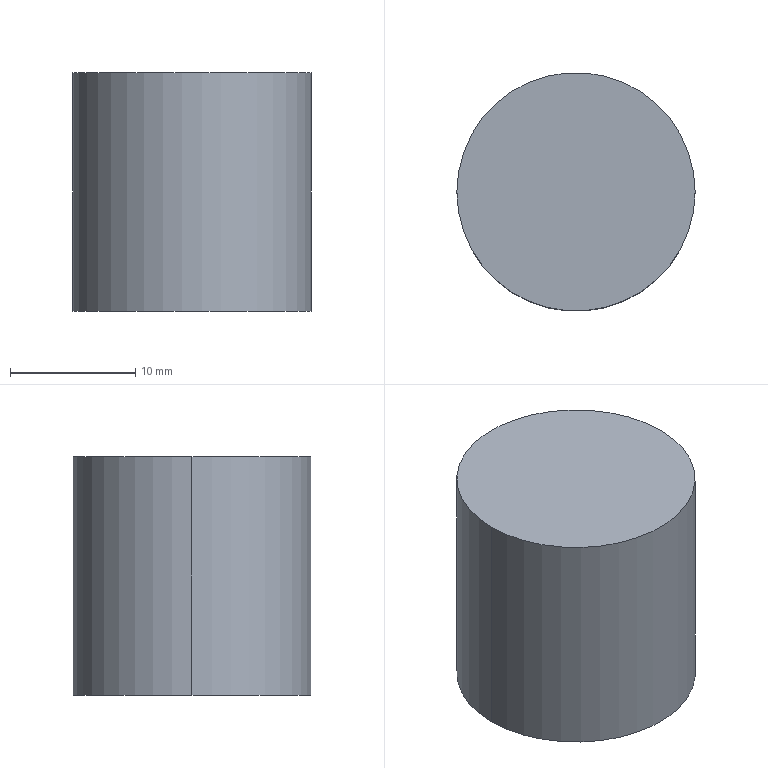Part | SolidWorks | features Extrusion 1 | 1 solid | 4 faces | box 19 x 19 x 19 mm | volume 5387 mm3 | cylinder 2 | plane 2 | commonest cylinder face diameters 19 x2
STEP:
#1=CARTESIAN_POINT('',(9.5,0.,19.));
#2=VERTEX_POINT('',#1);
#3=CARTESIAN_POINT('',(-9.5,0.,19.));
#4=VERTEX_POINT('',#3);
#5=CARTESIAN_POINT('',(0.,0.,19.));
#6=DIRECTION('',(0.,0.,1.));
#7=DIRECTION('',(1.,0.,0.));
#8=AXIS2_PLACEMENT_3D('',#5,#6,#7);
#9=CIRCLE('',#8,9.5);
#10=EDGE_CURVE('',#2,#4,#9,.T.);
#11=ORIENTED_EDGE('',*,*,#10,.F.);
#12=CARTESIAN_POINT('',(9.5,0.,0.));
#13=VERTEX_POINT('',#12);
#14=CARTESIAN_POINT('',(9.5,0.,19.));
#15=DIRECTION('',(0.,0.,-1.));
#16=VECTOR('',#15,1000.);
#17=LINE('',#14,#16);
#18=EDGE_CURVE('',#2,#13,#17,.T.);
#19=ORIENTED_EDGE('',*,*,#18,.T.);
#20=CARTESIAN_POINT('',(-9.5,0.,0.));
#21=VERTEX_POINT('',#20);
#22=CARTESIAN_POINT('',(0.,0.,0.));
#23=DIRECTION('',(0.,0.,1.));
#24=DIRECTION('',(1.,0.,0.));
#25=AXIS2_PLACEMENT_3D('',#22,#23,#24);
#26=CIRCLE('',#25,9.5);
#27=EDGE_CURVE('',#13,#21,#26,.T.);
#28=ORIENTED_EDGE('',*,*,#27,.T.);
#29=CARTESIAN_POINT('',(-9.5,0.,19.));
#30=DIRECTION('',(0.,0.,-1.));
#31=VECTOR('',#30,1000.);
#32=LINE('',#29,#31);
#33=EDGE_CURVE('',#4,#21,#32,.T.);
#34=ORIENTED_EDGE('',*,*,#33,.F.);
#35=EDGE_LOOP('',(#11,#19,#28,#34));
#36=FACE_OUTER_BOUND('',#35,.T.);
#37=CARTESIAN_POINT('',(0.,0.,19.));
#38=DIRECTION('',(0.,0.,-1.));
#39=DIRECTION('',(-1.,0.,0.));
#40=AXIS2_PLACEMENT_3D('',#37,#38,#39);
#41=CYLINDRICAL_SURFACE('',#40,9.5);
#42=ADVANCED_FACE('',(#36),#41,.T.);
#43=ORIENTED_EDGE('',*,*,#18,.F.);
#44=CARTESIAN_POINT('',(0.,0.,19.));
#45=DIRECTION('',(0.,0.,1.));
#46=DIRECTION('',(1.,0.,0.));
#47=AXIS2_PLACEMENT_3D('',#44,#45,#46);
#48=CIRCLE('',#47,9.5);
#49=EDGE_CURVE('',#4,#2,#48,.T.);
#50=ORIENTED_EDGE('',*,*,#49,.F.);
#51=ORIENTED_EDGE('',*,*,#33,.T.);
#52=CARTESIAN_POINT('',(0.,0.,0.));
#53=DIRECTION('',(0.,0.,1.));
#54=DIRECTION('',(1.,0.,0.));
#55=AXIS2_PLACEMENT_3D('',#52,#53,#54);
#56=CIRCLE('',#55,9.5);
#57=EDGE_CURVE('',#21,#13,#56,.T.);
#58=ORIENTED_EDGE('',*,*,#57,.T.);
#59=EDGE_LOOP('',(#43,#50,#51,#58));
#60=FACE_OUTER_BOUND('',#59,.T.);
#61=CARTESIAN_POINT('',(0.,0.,19.));
#62=DIRECTION('',(0.,0.,-1.));
#63=DIRECTION('',(-1.,0.,0.));
#64=AXIS2_PLACEMENT_3D('',#61,#62,#63);
#65=CYLINDRICAL_SURFACE('',#64,9.5);
#66=ADVANCED_FACE('',(#60),#65,.T.);
#67=ORIENTED_EDGE('',*,*,#49,.T.);
#68=ORIENTED_EDGE('',*,*,#10,.T.);
#69=EDGE_LOOP('',(#67,#68));
#70=FACE_OUTER_BOUND('',#69,.T.);
#71=CARTESIAN_POINT('',(0.,0.,19.));
#72=DIRECTION('',(0.,0.,1.));
#73=DIRECTION('',(1.,0.,0.));
#74=AXIS2_PLACEMENT_3D('',#71,#72,#73);
#75=PLANE('',#74);
#76=ADVANCED_FACE('',(#70),#75,.T.);
#77=ORIENTED_EDGE('',*,*,#57,.F.);
#78=ORIENTED_EDGE('',*,*,#27,.F.);
#79=EDGE_LOOP('',(#77,#78));
#80=FACE_OUTER_BOUND('',#79,.T.);
#81=CARTESIAN_POINT('',(0.,0.,0.));
#82=DIRECTION('',(0.,0.,1.));
#83=DIRECTION('',(1.,0.,0.));
#84=AXIS2_PLACEMENT_3D('',#81,#82,#83);
#85=PLANE('',#84);
#86=ADVANCED_FACE('',(#80),#85,.F.);
#87=CLOSED_SHELL('',(#42,#66,#76,#86));
#88=MANIFOLD_SOLID_BREP('',#87);
#89=CARTESIAN_POINT('',(0.,0.,0.));
#90=DIRECTION('',(0.,0.,1.));
#91=DIRECTION('',(1.,0.,0.));
#92=AXIS2_PLACEMENT_3D('',#89,#90,#91);
#93=(LENGTH_UNIT()NAMED_UNIT(*)SI_UNIT(.MILLI.,.METRE.));
#94=UNCERTAINTY_MEASURE_WITH_UNIT(LENGTH_MEASURE(0.00001),#93,'','');
#95=(NAMED_UNIT(*)PLANE_ANGLE_UNIT()SI_UNIT($,.RADIAN.));
#96=(NAMED_UNIT(*)SI_UNIT($,.STERADIAN.)SOLID_ANGLE_UNIT());
#97=(GEOMETRIC_REPRESENTATION_CONTEXT(3)GLOBAL_UNCERTAINTY_ASSIGNED_CONTEXT((#94))GLOBAL_UNIT_ASSIGNED_CONTEXT((#93,#95,#96))REPRESENTATION_CONTEXT('',''));
#98=ADVANCED_BREP_SHAPE_REPRESENTATION('',(#88,#92),#97);